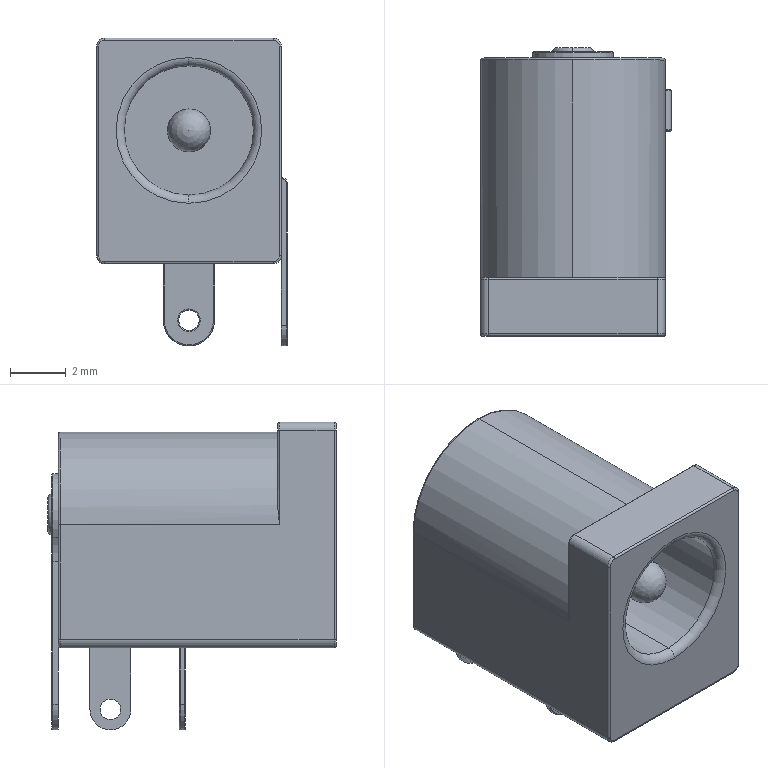Part | NX | features BREP 1 | 1 solid | 323 faces | box 6.836 x 10.327 x 11.025 mm | volume 376.134 mm3 | plane 147 | spline 98 | cylinder 44 | torus 33 | sphere 1 | commonest cylinder face diameters 0.147 x10 0.074 x8 0.735 x6 0.588 x4 1.838 x3 0.882 x2